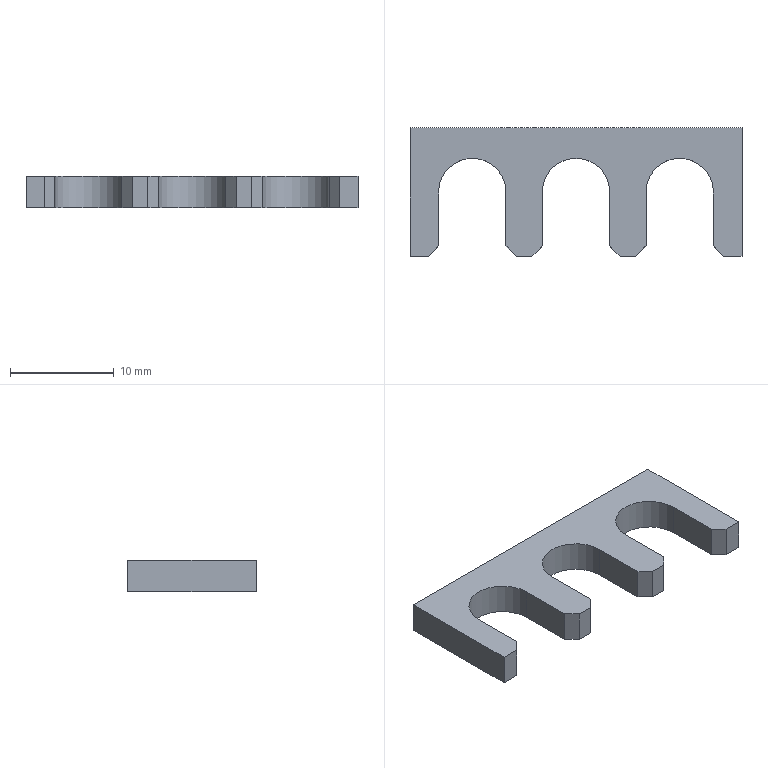Part | NX | features BREP 1 | 1 solid | 24 faces | box 32 x 12.4 x 3 mm | volume 669.376 mm3 | plane 21 | cylinder 3 | commonest cylinder face diameters 6.5 x3
STEP:
#1=CARTESIAN_POINT('',(-16.,0.,0.));
#2=VERTEX_POINT('',#1);
#3=CARTESIAN_POINT('',(-16.,-12.4,0.));
#4=VERTEX_POINT('',#3);
#5=CARTESIAN_POINT('',(-16.,-12.4,0.));
#6=DIRECTION('',(0.,-1.,0.));
#7=VECTOR('',#6,1000.);
#8=LINE('',#5,#7);
#9=EDGE_CURVE('',#2,#4,#8,.T.);
#10=ORIENTED_EDGE('',*,*,#9,.T.);
#11=CARTESIAN_POINT('',(-16.,-12.4,3.));
#12=VERTEX_POINT('',#11);
#13=CARTESIAN_POINT('',(-16.,-12.4,3.));
#14=DIRECTION('',(0.,0.,-1.));
#15=VECTOR('',#14,1000.);
#16=LINE('',#13,#15);
#17=EDGE_CURVE('',#12,#4,#16,.T.);
#18=ORIENTED_EDGE('',*,*,#17,.F.);
#19=CARTESIAN_POINT('',(-16.,0.,3.));
#20=VERTEX_POINT('',#19);
#21=CARTESIAN_POINT('',(-16.,-12.4,3.));
#22=DIRECTION('',(0.,-1.,0.));
#23=VECTOR('',#22,1000.);
#24=LINE('',#21,#23);
#25=EDGE_CURVE('',#20,#12,#24,.T.);
#26=ORIENTED_EDGE('',*,*,#25,.F.);
#27=CARTESIAN_POINT('',(-16.,0.,3.));
#28=DIRECTION('',(0.,0.,-1.));
#29=VECTOR('',#28,1000.);
#30=LINE('',#27,#29);
#31=EDGE_CURVE('',#20,#2,#30,.T.);
#32=ORIENTED_EDGE('',*,*,#31,.T.);
#33=EDGE_LOOP('',(#10,#18,#26,#32));
#34=FACE_BOUND('',#33,.T.);
#35=CARTESIAN_POINT('',(-16.,-12.4,3.));
#36=DIRECTION('',(1.,0.,0.));
#37=DIRECTION('',(0.,-1.,0.));
#38=AXIS2_PLACEMENT_3D('',#35,#36,#37);
#39=PLANE('',#38);
#40=ADVANCED_FACE('',(#34),#39,.F.);
#41=CARTESIAN_POINT('',(-14.25,-12.4,0.));
#42=VERTEX_POINT('',#41);
#43=CARTESIAN_POINT('',(-13.25,-12.4,0.));
#44=DIRECTION('',(1.,0.,0.));
#45=VECTOR('',#44,1000.);
#46=LINE('',#43,#45);
#47=EDGE_CURVE('',#4,#42,#46,.T.);
#48=ORIENTED_EDGE('',*,*,#47,.T.);
#49=CARTESIAN_POINT('',(-14.25,-12.4,3.));
#50=VERTEX_POINT('',#49);
#51=CARTESIAN_POINT('',(-14.25,-12.4,3.));
#52=DIRECTION('',(0.,0.,1.));
#53=VECTOR('',#52,1000.);
#54=LINE('',#51,#53);
#55=EDGE_CURVE('',#42,#50,#54,.T.);
#56=ORIENTED_EDGE('',*,*,#55,.T.);
#57=CARTESIAN_POINT('',(-13.25,-12.4,3.));
#58=DIRECTION('',(1.,0.,0.));
#59=VECTOR('',#58,1000.);
#60=LINE('',#57,#59);
#61=EDGE_CURVE('',#12,#50,#60,.T.);
#62=ORIENTED_EDGE('',*,*,#61,.F.);
#63=ORIENTED_EDGE('',*,*,#17,.T.);
#64=EDGE_LOOP('',(#48,#56,#62,#63));
#65=FACE_BOUND('',#64,.T.);
#66=CARTESIAN_POINT('',(-13.25,-12.4,3.));
#67=DIRECTION('',(0.,1.,0.));
#68=DIRECTION('',(0.,0.,-1.));
#69=AXIS2_PLACEMENT_3D('',#66,#67,#68);
#70=PLANE('',#69);
#71=ADVANCED_FACE('',(#65),#70,.F.);
#72=CARTESIAN_POINT('',(-13.25,-11.4,3.));
#73=VERTEX_POINT('',#72);
#74=CARTESIAN_POINT('',(-13.25,-6.2,3.));
#75=VERTEX_POINT('',#74);
#76=CARTESIAN_POINT('',(-13.25,-6.2,3.));
#77=DIRECTION('',(0.,1.,0.));
#78=VECTOR('',#77,1000.);
#79=LINE('',#76,#78);
#80=EDGE_CURVE('',#73,#75,#79,.T.);
#81=ORIENTED_EDGE('',*,*,#80,.F.);
#82=CARTESIAN_POINT('',(-13.25,-11.4,0.));
#83=VERTEX_POINT('',#82);
#84=CARTESIAN_POINT('',(-13.25,-11.4,3.));
#85=DIRECTION('',(0.,0.,-1.));
#86=VECTOR('',#85,1000.);
#87=LINE('',#84,#86);
#88=EDGE_CURVE('',#73,#83,#87,.T.);
#89=ORIENTED_EDGE('',*,*,#88,.T.);
#90=CARTESIAN_POINT('',(-13.25,-6.2,0.));
#91=VERTEX_POINT('',#90);
#92=CARTESIAN_POINT('',(-13.25,-6.2,0.));
#93=DIRECTION('',(0.,1.,0.));
#94=VECTOR('',#93,1000.);
#95=LINE('',#92,#94);
#96=EDGE_CURVE('',#83,#91,#95,.T.);
#97=ORIENTED_EDGE('',*,*,#96,.T.);
#98=CARTESIAN_POINT('',(-13.25,-6.2,3.));
#99=DIRECTION('',(0.,0.,-1.));
#100=VECTOR('',#99,1000.);
#101=LINE('',#98,#100);
#102=EDGE_CURVE('',#75,#91,#101,.T.);
#103=ORIENTED_EDGE('',*,*,#102,.F.);
#104=EDGE_LOOP('',(#81,#89,#97,#103));
#105=FACE_BOUND('',#104,.T.);
#106=CARTESIAN_POINT('',(-13.25,-6.2,3.));
#107=DIRECTION('',(-1.,0.,0.));
#108=DIRECTION('',(0.,0.,-1.));
#109=AXIS2_PLACEMENT_3D('',#106,#107,#108);
#110=PLANE('',#109);
#111=ADVANCED_FACE('',(#105),#110,.F.);
#112=CARTESIAN_POINT('',(-6.75,-6.2,0.));
#113=VERTEX_POINT('',#112);
#114=CARTESIAN_POINT('',(-10.,-6.2,0.));
#115=DIRECTION('',(0.,0.,-1.));
#116=DIRECTION('',(1.,0.,0.));
#117=AXIS2_PLACEMENT_3D('',#114,#115,#116);
#118=CIRCLE('',#117,3.25);
#119=EDGE_CURVE('',#91,#113,#118,.T.);
#120=ORIENTED_EDGE('',*,*,#119,.T.);
#121=CARTESIAN_POINT('',(-6.75,-6.2,3.));
#122=VERTEX_POINT('',#121);
#123=CARTESIAN_POINT('',(-6.75,-6.2,3.));
#124=DIRECTION('',(0.,0.,-1.));
#125=VECTOR('',#124,1000.);
#126=LINE('',#123,#125);
#127=EDGE_CURVE('',#122,#113,#126,.T.);
#128=ORIENTED_EDGE('',*,*,#127,.F.);
#129=CARTESIAN_POINT('',(-10.,-6.2,3.));
#130=DIRECTION('',(0.,0.,-1.));
#131=DIRECTION('',(1.,0.,0.));
#132=AXIS2_PLACEMENT_3D('',#129,#130,#131);
#133=CIRCLE('',#132,3.25);
#134=EDGE_CURVE('',#75,#122,#133,.T.);
#135=ORIENTED_EDGE('',*,*,#134,.F.);
#136=ORIENTED_EDGE('',*,*,#102,.T.);
#137=EDGE_LOOP('',(#120,#128,#135,#136));
#138=FACE_BOUND('',#137,.T.);
#139=CARTESIAN_POINT('',(-10.,-6.2,3.));
#140=DIRECTION('',(0.,0.,-1.));
#141=DIRECTION('',(1.,0.,0.));
#142=AXIS2_PLACEMENT_3D('',#139,#140,#141);
#143=CYLINDRICAL_SURFACE('',#142,3.25);
#144=ADVANCED_FACE('',(#138),#143,.F.);
#145=CARTESIAN_POINT('',(-6.75,-11.4,0.));
#146=VERTEX_POINT('',#145);
#147=CARTESIAN_POINT('',(-6.75,-12.4,0.));
#148=DIRECTION('',(0.,-1.,0.));
#149=VECTOR('',#148,1000.);
#150=LINE('',#147,#149);
#151=EDGE_CURVE('',#113,#146,#150,.T.);
#152=ORIENTED_EDGE('',*,*,#151,.T.);
#153=CARTESIAN_POINT('',(-6.75,-11.4,3.));
#154=VERTEX_POINT('',#153);
#155=CARTESIAN_POINT('',(-6.75,-11.4,3.));
#156=DIRECTION('',(0.,0.,1.));
#157=VECTOR('',#156,1000.);
#158=LINE('',#155,#157);
#159=EDGE_CURVE('',#146,#154,#158,.T.);
#160=ORIENTED_EDGE('',*,*,#159,.T.);
#161=CARTESIAN_POINT('',(-6.75,-12.4,3.));
#162=DIRECTION('',(0.,-1.,0.));
#163=VECTOR('',#162,1000.);
#164=LINE('',#161,#163);
#165=EDGE_CURVE('',#122,#154,#164,.T.);
#166=ORIENTED_EDGE('',*,*,#165,.F.);
#167=ORIENTED_EDGE('',*,*,#127,.T.);
#168=EDGE_LOOP('',(#152,#160,#166,#167));
#169=FACE_BOUND('',#168,.T.);
#170=CARTESIAN_POINT('',(-6.75,-12.4,3.));
#171=DIRECTION('',(1.,0.,0.));
#172=DIRECTION('',(0.,0.,1.));
#173=AXIS2_PLACEMENT_3D('',#170,#171,#172);
#174=PLANE('',#173);
#175=ADVANCED_FACE('',(#169),#174,.F.);
#176=CARTESIAN_POINT('',(-5.75,-12.4,0.));
#177=VERTEX_POINT('',#176);
#178=CARTESIAN_POINT('',(-4.25,-12.4,0.));
#179=VERTEX_POINT('',#178);
#180=CARTESIAN_POINT('',(-3.25,-12.4,0.));
#181=DIRECTION('',(1.,0.,0.));
#182=VECTOR('',#181,1000.);
#183=LINE('',#180,#182);
#184=EDGE_CURVE('',#177,#179,#183,.T.);
#185=ORIENTED_EDGE('',*,*,#184,.T.);
#186=CARTESIAN_POINT('',(-4.25,-12.4,3.));
#187=VERTEX_POINT('',#186);
#188=CARTESIAN_POINT('',(-4.25,-12.4,3.));
#189=DIRECTION('',(0.,0.,1.));
#190=VECTOR('',#189,1000.);
#191=LINE('',#188,#190);
#192=EDGE_CURVE('',#179,#187,#191,.T.);
#193=ORIENTED_EDGE('',*,*,#192,.T.);
#194=CARTESIAN_POINT('',(-5.75,-12.4,3.));
#195=VERTEX_POINT('',#194);
#196=CARTESIAN_POINT('',(-3.25,-12.4,3.));
#197=DIRECTION('',(1.,0.,0.));
#198=VECTOR('',#197,1000.);
#199=LINE('',#196,#198);
#200=EDGE_CURVE('',#195,#187,#199,.T.);
#201=ORIENTED_EDGE('',*,*,#200,.F.);
#202=CARTESIAN_POINT('',(-5.75,-12.4,3.));
#203=DIRECTION('',(0.,0.,-1.));
#204=VECTOR('',#203,1000.);
#205=LINE('',#202,#204);
#206=EDGE_CURVE('',#195,#177,#205,.T.);
#207=ORIENTED_EDGE('',*,*,#206,.T.);
#208=EDGE_LOOP('',(#185,#193,#201,#207));
#209=FACE_BOUND('',#208,.T.);
#210=CARTESIAN_POINT('',(-3.25,-12.4,3.));
#211=DIRECTION('',(0.,1.,0.));
#212=DIRECTION('',(0.,0.,-1.));
#213=AXIS2_PLACEMENT_3D('',#210,#211,#212);
#214=PLANE('',#213);
#215=ADVANCED_FACE('',(#209),#214,.F.);
#216=CARTESIAN_POINT('',(-3.25,-11.4,3.));
#217=VERTEX_POINT('',#216);
#218=CARTESIAN_POINT('',(-3.25,-6.2,3.));
#219=VERTEX_POINT('',#218);
#220=CARTESIAN_POINT('',(-3.25,-6.2,3.));
#221=DIRECTION('',(0.,1.,0.));
#222=VECTOR('',#221,1000.);
#223=LINE('',#220,#222);
#224=EDGE_CURVE('',#217,#219,#223,.T.);
#225=ORIENTED_EDGE('',*,*,#224,.F.);
#226=CARTESIAN_POINT('',(-3.25,-11.4,0.));
#227=VERTEX_POINT('',#226);
#228=CARTESIAN_POINT('',(-3.25,-11.4,3.));
#229=DIRECTION('',(0.,0.,-1.));
#230=VECTOR('',#229,1000.);
#231=LINE('',#228,#230);
#232=EDGE_CURVE('',#217,#227,#231,.T.);
#233=ORIENTED_EDGE('',*,*,#232,.T.);
#234=CARTESIAN_POINT('',(-3.25,-6.2,0.));
#235=VERTEX_POINT('',#234);
#236=CARTESIAN_POINT('',(-3.25,-6.2,0.));
#237=DIRECTION('',(0.,1.,0.));
#238=VECTOR('',#237,1000.);
#239=LINE('',#236,#238);
#240=EDGE_CURVE('',#227,#235,#239,.T.);
#241=ORIENTED_EDGE('',*,*,#240,.T.);
#242=CARTESIAN_POINT('',(-3.25,-6.2,3.));
#243=DIRECTION('',(0.,0.,-1.));
#244=VECTOR('',#243,1000.);
#245=LINE('',#242,#244);
#246=EDGE_CURVE('',#219,#235,#245,.T.);
#247=ORIENTED_EDGE('',*,*,#246,.F.);
#248=EDGE_LOOP('',(#225,#233,#241,#247));
#249=FACE_BOUND('',#248,.T.);
#250=CARTESIAN_POINT('',(-3.25,-6.2,3.));
#251=DIRECTION('',(-1.,0.,0.));
#252=DIRECTION('',(0.,1.,0.));
#253=AXIS2_PLACEMENT_3D('',#250,#251,#252);
#254=PLANE('',#253);
#255=ADVANCED_FACE('',(#249),#254,.F.);
#256=CARTESIAN_POINT('',(3.25,-6.2,0.));
#257=VERTEX_POINT('',#256);
#258=CARTESIAN_POINT('',(0.,-6.2,0.));
#259=DIRECTION('',(0.,0.,-1.));
#260=DIRECTION('',(1.,0.,0.));
#261=AXIS2_PLACEMENT_3D('',#258,#259,#260);
#262=CIRCLE('',#261,3.25);
#263=EDGE_CURVE('',#235,#257,#262,.T.);
#264=ORIENTED_EDGE('',*,*,#263,.T.);
#265=CARTESIAN_POINT('',(3.25,-6.2,3.));
#266=VERTEX_POINT('',#265);
#267=CARTESIAN_POINT('',(3.25,-6.2,3.));
#268=DIRECTION('',(0.,0.,-1.));
#269=VECTOR('',#268,1000.);
#270=LINE('',#267,#269);
#271=EDGE_CURVE('',#266,#257,#270,.T.);
#272=ORIENTED_EDGE('',*,*,#271,.F.);
#273=CARTESIAN_POINT('',(0.,-6.2,3.));
#274=DIRECTION('',(0.,0.,-1.));
#275=DIRECTION('',(1.,0.,0.));
#276=AXIS2_PLACEMENT_3D('',#273,#274,#275);
#277=CIRCLE('',#276,3.25);
#278=EDGE_CURVE('',#219,#266,#277,.T.);
#279=ORIENTED_EDGE('',*,*,#278,.F.);
#280=ORIENTED_EDGE('',*,*,#246,.T.);
#281=EDGE_LOOP('',(#264,#272,#279,#280));
#282=FACE_BOUND('',#281,.T.);
#283=CARTESIAN_POINT('',(0.,-6.2,3.));
#284=DIRECTION('',(0.,0.,-1.));
#285=DIRECTION('',(1.,0.,0.));
#286=AXIS2_PLACEMENT_3D('',#283,#284,#285);
#287=CYLINDRICAL_SURFACE('',#286,3.25);
#288=ADVANCED_FACE('',(#282),#287,.F.);
#289=CARTESIAN_POINT('',(3.25,-11.4,0.));
#290=VERTEX_POINT('',#289);
#291=CARTESIAN_POINT('',(3.25,-12.4,0.));
#292=DIRECTION('',(0.,-1.,0.));
#293=VECTOR('',#292,1000.);
#294=LINE('',#291,#293);
#295=EDGE_CURVE('',#257,#290,#294,.T.);
#296=ORIENTED_EDGE('',*,*,#295,.T.);
#297=CARTESIAN_POINT('',(3.25,-11.4,3.));
#298=VERTEX_POINT('',#297);
#299=CARTESIAN_POINT('',(3.25,-11.4,3.));
#300=DIRECTION('',(0.,0.,1.));
#301=VECTOR('',#300,1000.);
#302=LINE('',#299,#301);
#303=EDGE_CURVE('',#290,#298,#302,.T.);
#304=ORIENTED_EDGE('',*,*,#303,.T.);
#305=CARTESIAN_POINT('',(3.25,-12.4,3.));
#306=DIRECTION('',(0.,-1.,0.));
#307=VECTOR('',#306,1000.);
#308=LINE('',#305,#307);
#309=EDGE_CURVE('',#266,#298,#308,.T.);
#310=ORIENTED_EDGE('',*,*,#309,.F.);
#311=ORIENTED_EDGE('',*,*,#271,.T.);
#312=EDGE_LOOP('',(#296,#304,#310,#311));
#313=FACE_BOUND('',#312,.T.);
#314=CARTESIAN_POINT('',(3.25,-12.4,3.));
#315=DIRECTION('',(1.,0.,0.));
#316=DIRECTION('',(0.,0.,1.));
#317=AXIS2_PLACEMENT_3D('',#314,#315,#316);
#318=PLANE('',#317);
#319=ADVANCED_FACE('',(#313),#318,.F.);
#320=CARTESIAN_POINT('',(4.25,-12.4,0.));
#321=VERTEX_POINT('',#320);
#322=CARTESIAN_POINT('',(5.75,-12.4,0.));
#323=VERTEX_POINT('',#322);
#324=CARTESIAN_POINT('',(6.75,-12.4,0.));
#325=DIRECTION('',(1.,0.,0.));
#326=VECTOR('',#325,1000.);
#327=LINE('',#324,#326);
#328=EDGE_CURVE('',#321,#323,#327,.T.);
#329=ORIENTED_EDGE('',*,*,#328,.T.);
#330=CARTESIAN_POINT('',(5.75,-12.4,3.));
#331=VERTEX_POINT('',#330);
#332=CARTESIAN_POINT('',(5.75,-12.4,3.));
#333=DIRECTION('',(0.,0.,1.));
#334=VECTOR('',#333,1000.);
#335=LINE('',#332,#334);
#336=EDGE_CURVE('',#323,#331,#335,.T.);
#337=ORIENTED_EDGE('',*,*,#336,.T.);
#338=CARTESIAN_POINT('',(4.25,-12.4,3.));
#339=VERTEX_POINT('',#338);
#340=CARTESIAN_POINT('',(6.75,-12.4,3.));
#341=DIRECTION('',(1.,0.,0.));
#342=VECTOR('',#341,1000.);
#343=LINE('',#340,#342);
#344=EDGE_CURVE('',#339,#331,#343,.T.);
#345=ORIENTED_EDGE('',*,*,#344,.F.);
#346=CARTESIAN_POINT('',(4.25,-12.4,3.));
#347=DIRECTION('',(0.,0.,-1.));
#348=VECTOR('',#347,1000.);
#349=LINE('',#346,#348);
#350=EDGE_CURVE('',#339,#321,#349,.T.);
#351=ORIENTED_EDGE('',*,*,#350,.T.);
#352=EDGE_LOOP('',(#329,#337,#345,#351));
#353=FACE_BOUND('',#352,.T.);
#354=CARTESIAN_POINT('',(6.75,-12.4,3.));
#355=DIRECTION('',(0.,1.,0.));
#356=DIRECTION('',(0.,0.,-1.));
#357=AXIS2_PLACEMENT_3D('',#354,#355,#356);
#358=PLANE('',#357);
#359=ADVANCED_FACE('',(#353),#358,.F.);
#360=CARTESIAN_POINT('',(6.75,-11.4,3.));
#361=VERTEX_POINT('',#360);
#362=CARTESIAN_POINT('',(6.75,-6.2,3.));
#363=VERTEX_POINT('',#362);
#364=CARTESIAN_POINT('',(6.75,-6.2,3.));
#365=DIRECTION('',(0.,1.,0.));
#366=VECTOR('',#365,1000.);
#367=LINE('',#364,#366);
#368=EDGE_CURVE('',#361,#363,#367,.T.);
#369=ORIENTED_EDGE('',*,*,#368,.F.);
#370=CARTESIAN_POINT('',(6.75,-11.4,0.));
#371=VERTEX_POINT('',#370);
#372=CARTESIAN_POINT('',(6.75,-11.4,3.));
#373=DIRECTION('',(0.,0.,-1.));
#374=VECTOR('',#373,1000.);
#375=LINE('',#372,#374);
#376=EDGE_CURVE('',#361,#371,#375,.T.);
#377=ORIENTED_EDGE('',*,*,#376,.T.);
#378=CARTESIAN_POINT('',(6.75,-6.2,0.));
#379=VERTEX_POINT('',#378);
#380=CARTESIAN_POINT('',(6.75,-6.2,0.));
#381=DIRECTION('',(0.,1.,0.));
#382=VECTOR('',#381,1000.);
#383=LINE('',#380,#382);
#384=EDGE_CURVE('',#371,#379,#383,.T.);
#385=ORIENTED_EDGE('',*,*,#384,.T.);
#386=CARTESIAN_POINT('',(6.75,-6.2,3.));
#387=DIRECTION('',(0.,0.,-1.));
#388=VECTOR('',#387,1000.);
#389=LINE('',#386,#388);
#390=EDGE_CURVE('',#363,#379,#389,.T.);
#391=ORIENTED_EDGE('',*,*,#390,.F.);
#392=EDGE_LOOP('',(#369,#377,#385,#391));
#393=FACE_BOUND('',#392,.T.);
#394=CARTESIAN_POINT('',(6.75,-6.2,3.));
#395=DIRECTION('',(-1.,0.,0.));
#396=DIRECTION('',(0.,0.,-1.));
#397=AXIS2_PLACEMENT_3D('',#394,#395,#396);
#398=PLANE('',#397);
#399=ADVANCED_FACE('',(#393),#398,.F.);
#400=CARTESIAN_POINT('',(13.25,-6.2,0.));
#401=VERTEX_POINT('',#400);
#402=CARTESIAN_POINT('',(10.,-6.2,0.));
#403=DIRECTION('',(0.,0.,-1.));
#404=DIRECTION('',(1.,0.,0.));
#405=AXIS2_PLACEMENT_3D('',#402,#403,#404);
#406=CIRCLE('',#405,3.25);
#407=EDGE_CURVE('',#379,#401,#406,.T.);
#408=ORIENTED_EDGE('',*,*,#407,.T.);
#409=CARTESIAN_POINT('',(13.25,-6.2,3.));
#410=VERTEX_POINT('',#409);
#411=CARTESIAN_POINT('',(13.25,-6.2,3.));
#412=DIRECTION('',(0.,0.,-1.));
#413=VECTOR('',#412,1000.);
#414=LINE('',#411,#413);
#415=EDGE_CURVE('',#410,#401,#414,.T.);
#416=ORIENTED_EDGE('',*,*,#415,.F.);
#417=CARTESIAN_POINT('',(10.,-6.2,3.));
#418=DIRECTION('',(0.,0.,-1.));
#419=DIRECTION('',(1.,0.,0.));
#420=AXIS2_PLACEMENT_3D('',#417,#418,#419);
#421=CIRCLE('',#420,3.25);
#422=EDGE_CURVE('',#363,#410,#421,.T.);
#423=ORIENTED_EDGE('',*,*,#422,.F.);
#424=ORIENTED_EDGE('',*,*,#390,.T.);
#425=EDGE_LOOP('',(#408,#416,#423,#424));
#426=FACE_BOUND('',#425,.T.);
#427=CARTESIAN_POINT('',(10.,-6.2,3.));
#428=DIRECTION('',(0.,0.,-1.));
#429=DIRECTION('',(1.,0.,0.));
#430=AXIS2_PLACEMENT_3D('',#427,#428,#429);
#431=CYLINDRICAL_SURFACE('',#430,3.25);
#432=ADVANCED_FACE('',(#426),#431,.F.);
#433=CARTESIAN_POINT('',(13.25,-11.4,0.));
#434=VERTEX_POINT('',#433);
#435=CARTESIAN_POINT('',(13.25,-12.4,0.));
#436=DIRECTION('',(0.,-1.,0.));
#437=VECTOR('',#436,1000.);
#438=LINE('',#435,#437);
#439=EDGE_CURVE('',#401,#434,#438,.T.);
#440=ORIENTED_EDGE('',*,*,#439,.T.);
#441=CARTESIAN_POINT('',(13.25,-11.4,3.));
#442=VERTEX_POINT('',#441);
#443=CARTESIAN_POINT('',(13.25,-11.4,3.));
#444=DIRECTION('',(0.,0.,1.));
#445=VECTOR('',#444,1000.);
#446=LINE('',#443,#445);
#447=EDGE_CURVE('',#434,#442,#446,.T.);
#448=ORIENTED_EDGE('',*,*,#447,.T.);
#449=CARTESIAN_POINT('',(13.25,-12.4,3.));
#450=DIRECTION('',(0.,-1.,0.));
#451=VECTOR('',#450,1000.);
#452=LINE('',#449,#451);
#453=EDGE_CURVE('',#410,#442,#452,.T.);
#454=ORIENTED_EDGE('',*,*,#453,.F.);
#455=ORIENTED_EDGE('',*,*,#415,.T.);
#456=EDGE_LOOP('',(#440,#448,#454,#455));
#457=FACE_BOUND('',#456,.T.);
#458=CARTESIAN_POINT('',(13.25,-12.4,3.));
#459=DIRECTION('',(1.,0.,0.));
#460=DIRECTION('',(0.,-1.,0.));
#461=AXIS2_PLACEMENT_3D('',#458,#459,#460);
#462=PLANE('',#461);
#463=ADVANCED_FACE('',(#457),#462,.F.);
#464=CARTESIAN_POINT('',(14.25,-12.4,3.));
#465=VERTEX_POINT('',#464);
#466=CARTESIAN_POINT('',(16.,-12.4,3.));
#467=VERTEX_POINT('',#466);
#468=CARTESIAN_POINT('',(16.,-12.4,3.));
#469=DIRECTION('',(1.,0.,0.));
#470=VECTOR('',#469,1000.);
#471=LINE('',#468,#470);
#472=EDGE_CURVE('',#465,#467,#471,.T.);
#473=ORIENTED_EDGE('',*,*,#472,.F.);
#474=CARTESIAN_POINT('',(14.25,-12.4,0.));
#475=VERTEX_POINT('',#474);
#476=CARTESIAN_POINT('',(14.25,-12.4,3.));
#477=DIRECTION('',(0.,0.,-1.));
#478=VECTOR('',#477,1000.);
#479=LINE('',#476,#478);
#480=EDGE_CURVE('',#465,#475,#479,.T.);
#481=ORIENTED_EDGE('',*,*,#480,.T.);
#482=CARTESIAN_POINT('',(16.,-12.4,0.));
#483=VERTEX_POINT('',#482);
#484=CARTESIAN_POINT('',(16.,-12.4,0.));
#485=DIRECTION('',(1.,0.,0.));
#486=VECTOR('',#485,1000.);
#487=LINE('',#484,#486);
#488=EDGE_CURVE('',#475,#483,#487,.T.);
#489=ORIENTED_EDGE('',*,*,#488,.T.);
#490=CARTESIAN_POINT('',(16.,-12.4,3.));
#491=DIRECTION('',(0.,0.,-1.));
#492=VECTOR('',#491,1000.);
#493=LINE('',#490,#492);
#494=EDGE_CURVE('',#467,#483,#493,.T.);
#495=ORIENTED_EDGE('',*,*,#494,.F.);
#496=EDGE_LOOP('',(#473,#481,#489,#495));
#497=FACE_BOUND('',#496,.T.);
#498=CARTESIAN_POINT('',(16.,-12.4,3.));
#499=DIRECTION('',(0.,1.,0.));
#500=DIRECTION('',(0.,0.,-1.));
#501=AXIS2_PLACEMENT_3D('',#498,#499,#500);
#502=PLANE('',#501);
#503=ADVANCED_FACE('',(#497),#502,.F.);
#504=CARTESIAN_POINT('',(16.,0.,0.));
#505=VERTEX_POINT('',#504);
#506=CARTESIAN_POINT('',(16.,0.,0.));
#507=DIRECTION('',(0.,1.,0.));
#508=VECTOR('',#507,1000.);
#509=LINE('',#506,#508);
#510=EDGE_CURVE('',#483,#505,#509,.T.);
#511=ORIENTED_EDGE('',*,*,#510,.T.);
#512=CARTESIAN_POINT('',(16.,0.,3.));
#513=VERTEX_POINT('',#512);
#514=CARTESIAN_POINT('',(16.,0.,3.));
#515=DIRECTION('',(0.,0.,-1.));
#516=VECTOR('',#515,1000.);
#517=LINE('',#514,#516);
#518=EDGE_CURVE('',#513,#505,#517,.T.);
#519=ORIENTED_EDGE('',*,*,#518,.F.);
#520=CARTESIAN_POINT('',(16.,0.,3.));
#521=DIRECTION('',(0.,1.,0.));
#522=VECTOR('',#521,1000.);
#523=LINE('',#520,#522);
#524=EDGE_CURVE('',#467,#513,#523,.T.);
#525=ORIENTED_EDGE('',*,*,#524,.F.);
#526=ORIENTED_EDGE('',*,*,#494,.T.);
#527=EDGE_LOOP('',(#511,#519,#525,#526));
#528=FACE_BOUND('',#527,.T.);
#529=CARTESIAN_POINT('',(16.,0.,3.));
#530=DIRECTION('',(-1.,0.,0.));
#531=DIRECTION('',(0.,1.,0.));
#532=AXIS2_PLACEMENT_3D('',#529,#530,#531);
#533=PLANE('',#532);
#534=ADVANCED_FACE('',(#528),#533,.F.);
#535=CARTESIAN_POINT('',(-16.,0.,0.));
#536=DIRECTION('',(-1.,0.,0.));
#537=VECTOR('',#536,1000.);
#538=LINE('',#535,#537);
#539=EDGE_CURVE('',#505,#2,#538,.T.);
#540=ORIENTED_EDGE('',*,*,#539,.T.);
#541=ORIENTED_EDGE('',*,*,#31,.F.);
#542=CARTESIAN_POINT('',(-16.,0.,3.));
#543=DIRECTION('',(-1.,0.,0.));
#544=VECTOR('',#543,1000.);
#545=LINE('',#542,#544);
#546=EDGE_CURVE('',#513,#20,#545,.T.);
#547=ORIENTED_EDGE('',*,*,#546,.F.);
#548=ORIENTED_EDGE('',*,*,#518,.T.);
#549=EDGE_LOOP('',(#540,#541,#547,#548));
#550=FACE_BOUND('',#549,.T.);
#551=CARTESIAN_POINT('',(-16.,0.,3.));
#552=DIRECTION('',(0.,-1.,0.));
#553=DIRECTION('',(-1.,0.,0.));
#554=AXIS2_PLACEMENT_3D('',#551,#552,#553);
#555=PLANE('',#554);
#556=ADVANCED_FACE('',(#550),#555,.F.);
#557=ORIENTED_EDGE('',*,*,#61,.T.);
#558=CARTESIAN_POINT('',(0.975,2.825,3.));
#559=DIRECTION('',(0.7071,0.7071,0.));
#560=VECTOR('',#559,1000.);
#561=LINE('',#558,#560);
#562=EDGE_CURVE('',#50,#73,#561,.T.);
#563=ORIENTED_EDGE('',*,*,#562,.T.);
#564=ORIENTED_EDGE('',*,*,#80,.T.);
#565=ORIENTED_EDGE('',*,*,#134,.T.);
#566=ORIENTED_EDGE('',*,*,#165,.T.);
#567=CARTESIAN_POINT('',(-0.975,-17.175,3.));
#568=DIRECTION('',(0.7071,-0.7071,0.));
#569=VECTOR('',#568,1000.);
#570=LINE('',#567,#569);
#571=EDGE_CURVE('',#154,#195,#570,.T.);
#572=ORIENTED_EDGE('',*,*,#571,.T.);
#573=ORIENTED_EDGE('',*,*,#200,.T.);
#574=CARTESIAN_POINT('',(5.975,-2.175,3.));
#575=DIRECTION('',(0.7071,0.7071,0.));
#576=VECTOR('',#575,1000.);
#577=LINE('',#574,#576);
#578=EDGE_CURVE('',#187,#217,#577,.T.);
#579=ORIENTED_EDGE('',*,*,#578,.T.);
#580=ORIENTED_EDGE('',*,*,#224,.T.);
#581=ORIENTED_EDGE('',*,*,#278,.T.);
#582=ORIENTED_EDGE('',*,*,#309,.T.);
#583=CARTESIAN_POINT('',(4.025,-12.175,3.));
#584=DIRECTION('',(0.7071,-0.7071,0.));
#585=VECTOR('',#584,1000.);
#586=LINE('',#583,#585);
#587=EDGE_CURVE('',#298,#339,#586,.T.);
#588=ORIENTED_EDGE('',*,*,#587,.T.);
#589=ORIENTED_EDGE('',*,*,#344,.T.);
#590=CARTESIAN_POINT('',(10.975,-7.175,3.));
#591=DIRECTION('',(0.7071,0.7071,0.));
#592=VECTOR('',#591,1000.);
#593=LINE('',#590,#592);
#594=EDGE_CURVE('',#331,#361,#593,.T.);
#595=ORIENTED_EDGE('',*,*,#594,.T.);
#596=ORIENTED_EDGE('',*,*,#368,.T.);
#597=ORIENTED_EDGE('',*,*,#422,.T.);
#598=ORIENTED_EDGE('',*,*,#453,.T.);
#599=CARTESIAN_POINT('',(9.025,-7.175,3.));
#600=DIRECTION('',(0.7071,-0.7071,0.));
#601=VECTOR('',#600,1000.);
#602=LINE('',#599,#601);
#603=EDGE_CURVE('',#442,#465,#602,.T.);
#604=ORIENTED_EDGE('',*,*,#603,.T.);
#605=ORIENTED_EDGE('',*,*,#472,.T.);
#606=ORIENTED_EDGE('',*,*,#524,.T.);
#607=ORIENTED_EDGE('',*,*,#546,.T.);
#608=ORIENTED_EDGE('',*,*,#25,.T.);
#609=EDGE_LOOP('',(#557,#563,#564,#565,#566,#572,#573,#579,#580,#581,#582,#588,#589,#595,#596,#597,#598,#604,#605,#606,#607,#608));
#610=FACE_BOUND('',#609,.T.);
#611=CARTESIAN_POINT('',(10.,-6.2,3.));
#612=DIRECTION('',(0.,0.,1.));
#613=DIRECTION('',(-1.,0.,0.));
#614=AXIS2_PLACEMENT_3D('',#611,#612,#613);
#615=PLANE('',#614);
#616=ADVANCED_FACE('',(#610),#615,.T.);
#617=ORIENTED_EDGE('',*,*,#96,.F.);
#618=CARTESIAN_POINT('',(-13.25,-11.4,0.));
#619=DIRECTION('',(-0.7071,-0.7071,0.));
#620=VECTOR('',#619,1000.);
#621=LINE('',#618,#620);
#622=EDGE_CURVE('',#83,#42,#621,.T.);
#623=ORIENTED_EDGE('',*,*,#622,.T.);
#624=ORIENTED_EDGE('',*,*,#47,.F.);
#625=ORIENTED_EDGE('',*,*,#9,.F.);
#626=ORIENTED_EDGE('',*,*,#539,.F.);
#627=ORIENTED_EDGE('',*,*,#510,.F.);
#628=ORIENTED_EDGE('',*,*,#488,.F.);
#629=CARTESIAN_POINT('',(14.25,-12.4,0.));
#630=DIRECTION('',(-0.7071,0.7071,0.));
#631=VECTOR('',#630,1000.);
#632=LINE('',#629,#631);
#633=EDGE_CURVE('',#475,#434,#632,.T.);
#634=ORIENTED_EDGE('',*,*,#633,.T.);
#635=ORIENTED_EDGE('',*,*,#439,.F.);
#636=ORIENTED_EDGE('',*,*,#407,.F.);
#637=ORIENTED_EDGE('',*,*,#384,.F.);
#638=CARTESIAN_POINT('',(6.75,-11.4,0.));
#639=DIRECTION('',(-0.7071,-0.7071,0.));
#640=VECTOR('',#639,1000.);
#641=LINE('',#638,#640);
#642=EDGE_CURVE('',#371,#323,#641,.T.);
#643=ORIENTED_EDGE('',*,*,#642,.T.);
#644=ORIENTED_EDGE('',*,*,#328,.F.);
#645=CARTESIAN_POINT('',(4.25,-12.4,0.));
#646=DIRECTION('',(-0.7071,0.7071,0.));
#647=VECTOR('',#646,1000.);
#648=LINE('',#645,#647);
#649=EDGE_CURVE('',#321,#290,#648,.T.);
#650=ORIENTED_EDGE('',*,*,#649,.T.);
#651=ORIENTED_EDGE('',*,*,#295,.F.);
#652=ORIENTED_EDGE('',*,*,#263,.F.);
#653=ORIENTED_EDGE('',*,*,#240,.F.);
#654=CARTESIAN_POINT('',(-3.25,-11.4,0.));
#655=DIRECTION('',(-0.7071,-0.7071,0.));
#656=VECTOR('',#655,1000.);
#657=LINE('',#654,#656);
#658=EDGE_CURVE('',#227,#179,#657,.T.);
#659=ORIENTED_EDGE('',*,*,#658,.T.);
#660=ORIENTED_EDGE('',*,*,#184,.F.);
#661=CARTESIAN_POINT('',(-5.75,-12.4,0.));
#662=DIRECTION('',(-0.7071,0.7071,0.));
#663=VECTOR('',#662,1000.);
#664=LINE('',#661,#663);
#665=EDGE_CURVE('',#177,#146,#664,.T.);
#666=ORIENTED_EDGE('',*,*,#665,.T.);
#667=ORIENTED_EDGE('',*,*,#151,.F.);
#668=ORIENTED_EDGE('',*,*,#119,.F.);
#669=EDGE_LOOP('',(#617,#623,#624,#625,#626,#627,#628,#634,#635,#636,#637,#643,#644,#650,#651,#652,#653,#659,#660,#666,#667,#668));
#670=FACE_BOUND('',#669,.T.);
#671=CARTESIAN_POINT('',(10.,-6.2,0.));
#672=DIRECTION('',(0.,0.,1.));
#673=DIRECTION('',(-1.,0.,0.));
#674=AXIS2_PLACEMENT_3D('',#671,#672,#673);
#675=PLANE('',#674);
#676=ADVANCED_FACE('',(#670),#675,.F.);
#677=ORIENTED_EDGE('',*,*,#562,.F.);
#678=ORIENTED_EDGE('',*,*,#55,.F.);
#679=ORIENTED_EDGE('',*,*,#622,.F.);
#680=ORIENTED_EDGE('',*,*,#88,.F.);
#681=EDGE_LOOP('',(#677,#678,#679,#680));
#682=FACE_BOUND('',#681,.T.);
#683=CARTESIAN_POINT('',(-13.25,-11.4,3.));
#684=DIRECTION('',(-0.7071,0.7071,0.));
#685=DIRECTION('',(0.,0.,1.));
#686=AXIS2_PLACEMENT_3D('',#683,#684,#685);
#687=PLANE('',#686);
#688=ADVANCED_FACE('',(#682),#687,.F.);
#689=ORIENTED_EDGE('',*,*,#603,.F.);
#690=ORIENTED_EDGE('',*,*,#447,.F.);
#691=ORIENTED_EDGE('',*,*,#633,.F.);
#692=ORIENTED_EDGE('',*,*,#480,.F.);
#693=EDGE_LOOP('',(#689,#690,#691,#692));
#694=FACE_BOUND('',#693,.T.);
#695=CARTESIAN_POINT('',(14.25,-12.4,3.));
#696=DIRECTION('',(0.7071,0.7071,0.));
#697=DIRECTION('',(0.,0.,1.));
#698=AXIS2_PLACEMENT_3D('',#695,#696,#697);
#699=PLANE('',#698);
#700=ADVANCED_FACE('',(#694),#699,.F.);
#701=ORIENTED_EDGE('',*,*,#594,.F.);
#702=ORIENTED_EDGE('',*,*,#336,.F.);
#703=ORIENTED_EDGE('',*,*,#642,.F.);
#704=ORIENTED_EDGE('',*,*,#376,.F.);
#705=EDGE_LOOP('',(#701,#702,#703,#704));
#706=FACE_BOUND('',#705,.T.);
#707=CARTESIAN_POINT('',(6.75,-11.4,3.));
#708=DIRECTION('',(-0.7071,0.7071,0.));
#709=DIRECTION('',(0.,0.,1.));
#710=AXIS2_PLACEMENT_3D('',#707,#708,#709);
#711=PLANE('',#710);
#712=ADVANCED_FACE('',(#706),#711,.F.);
#713=ORIENTED_EDGE('',*,*,#587,.F.);
#714=ORIENTED_EDGE('',*,*,#303,.F.);
#715=ORIENTED_EDGE('',*,*,#649,.F.);
#716=ORIENTED_EDGE('',*,*,#350,.F.);
#717=EDGE_LOOP('',(#713,#714,#715,#716));
#718=FACE_BOUND('',#717,.T.);
#719=CARTESIAN_POINT('',(4.25,-12.4,3.));
#720=DIRECTION('',(0.7071,0.7071,0.));
#721=DIRECTION('',(0.,0.,1.));
#722=AXIS2_PLACEMENT_3D('',#719,#720,#721);
#723=PLANE('',#722);
#724=ADVANCED_FACE('',(#718),#723,.F.);
#725=ORIENTED_EDGE('',*,*,#578,.F.);
#726=ORIENTED_EDGE('',*,*,#192,.F.);
#727=ORIENTED_EDGE('',*,*,#658,.F.);
#728=ORIENTED_EDGE('',*,*,#232,.F.);
#729=EDGE_LOOP('',(#725,#726,#727,#728));
#730=FACE_BOUND('',#729,.T.);
#731=CARTESIAN_POINT('',(-3.25,-11.4,3.));
#732=DIRECTION('',(-0.7071,0.7071,0.));
#733=DIRECTION('',(0.,0.,1.));
#734=AXIS2_PLACEMENT_3D('',#731,#732,#733);
#735=PLANE('',#734);
#736=ADVANCED_FACE('',(#730),#735,.F.);
#737=ORIENTED_EDGE('',*,*,#571,.F.);
#738=ORIENTED_EDGE('',*,*,#159,.F.);
#739=ORIENTED_EDGE('',*,*,#665,.F.);
#740=ORIENTED_EDGE('',*,*,#206,.F.);
#741=EDGE_LOOP('',(#737,#738,#739,#740));
#742=FACE_BOUND('',#741,.T.);
#743=CARTESIAN_POINT('',(-5.75,-12.4,3.));
#744=DIRECTION('',(0.7071,0.7071,0.));
#745=DIRECTION('',(0.,0.,1.));
#746=AXIS2_PLACEMENT_3D('',#743,#744,#745);
#747=PLANE('',#746);
#748=ADVANCED_FACE('',(#742),#747,.F.);
#749=CLOSED_SHELL('',(#40,#71,#111,#144,#175,#215,#255,#288,#319,#359,#399,#432,#463,#503,#534,#556,#616,#676,#688,#700,#712,#724,#736,#748));
#750=MANIFOLD_SOLID_BREP('',#749);
#751=(LENGTH_UNIT()NAMED_UNIT(*)SI_UNIT(.MILLI.,.METRE.));
#752=UNCERTAINTY_MEASURE_WITH_UNIT(LENGTH_MEASURE(0.00001),#751,'','');
#753=(NAMED_UNIT(*)PLANE_ANGLE_UNIT()SI_UNIT($,.RADIAN.));
#754=(NAMED_UNIT(*)SI_UNIT($,.STERADIAN.)SOLID_ANGLE_UNIT());
#755=(GEOMETRIC_REPRESENTATION_CONTEXT(3)GLOBAL_UNCERTAINTY_ASSIGNED_CONTEXT((#752))GLOBAL_UNIT_ASSIGNED_CONTEXT((#751,#753,#754))REPRESENTATION_CONTEXT('',''));
#756=ADVANCED_BREP_SHAPE_REPRESENTATION('',(#750),#755);